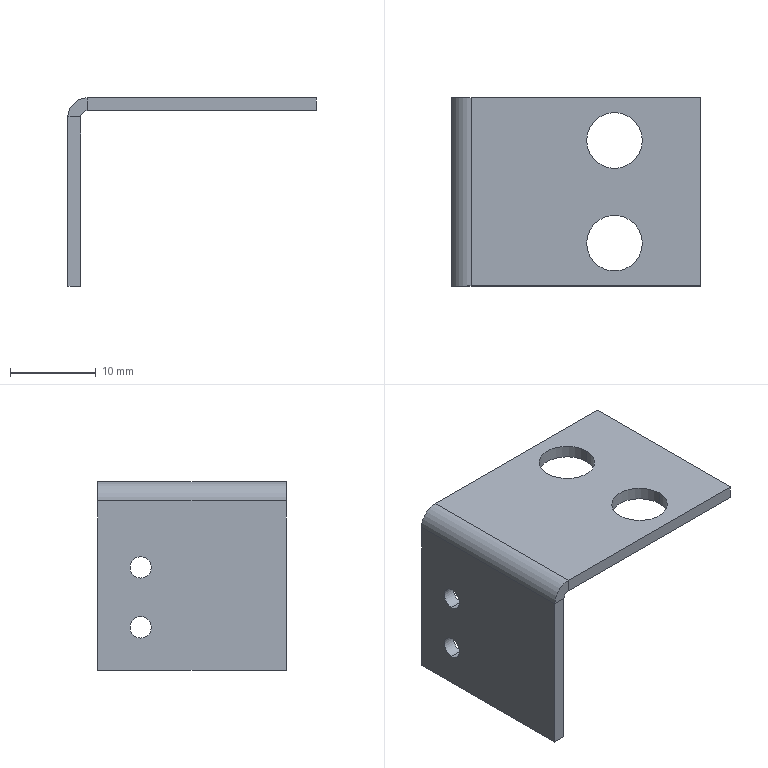Part | SolidWorks | features 3DProfileFeature 1, EdgeFlange 1, FlatPattern 1, HoleWzd 1, SMBaseFlange 1, SheetMetal 1 | 1 solid | 22 faces | box 29 x 22 x 22 mm | volume 1498 mm3 | plane 12 | cylinder 10 | commonest cylinder face diameters 2.5 x4 6.5 x4 1.473 x1 4.473 x1
STEP:
#1=CARTESIAN_POINT('',(-13.,6.,-11.25));
#2=VERTEX_POINT('',#1);
#3=CARTESIAN_POINT('',(-13.,6.,-8.75));
#4=VERTEX_POINT('',#3);
#5=CARTESIAN_POINT('',(-13.,6.,-10.));
#6=DIRECTION('',(-1.,0.,0.));
#7=DIRECTION('',(0.,0.,1.));
#8=AXIS2_PLACEMENT_3D('',#5,#6,#7);
#9=CIRCLE('',#8,1.25);
#10=EDGE_CURVE('',#2,#4,#9,.T.);
#11=ORIENTED_EDGE('',*,*,#10,.F.);
#12=CARTESIAN_POINT('',(-14.5,6.,-11.25));
#13=VERTEX_POINT('',#12);
#14=CARTESIAN_POINT('',(-14.5,6.,-11.25));
#15=DIRECTION('',(-1.,0.,0.));
#16=VECTOR('',#15,1000.);
#17=LINE('',#14,#16);
#18=EDGE_CURVE('',#2,#13,#17,.T.);
#19=ORIENTED_EDGE('',*,*,#18,.T.);
#20=CARTESIAN_POINT('',(-14.5,6.,-8.75));
#21=VERTEX_POINT('',#20);
#22=CARTESIAN_POINT('',(-14.5,6.,-10.));
#23=DIRECTION('',(-1.,0.,0.));
#24=DIRECTION('',(0.,0.,1.));
#25=AXIS2_PLACEMENT_3D('',#22,#23,#24);
#26=CIRCLE('',#25,1.25);
#27=EDGE_CURVE('',#13,#21,#26,.T.);
#28=ORIENTED_EDGE('',*,*,#27,.T.);
#29=CARTESIAN_POINT('',(-14.5,6.,-8.75));
#30=DIRECTION('',(-1.,0.,0.));
#31=VECTOR('',#30,1000.);
#32=LINE('',#29,#31);
#33=EDGE_CURVE('',#4,#21,#32,.T.);
#34=ORIENTED_EDGE('',*,*,#33,.F.);
#35=EDGE_LOOP('',(#11,#19,#28,#34));
#36=FACE_OUTER_BOUND('',#35,.T.);
#37=CARTESIAN_POINT('',(-14.5,6.,-10.));
#38=DIRECTION('',(-1.,0.,0.));
#39=DIRECTION('',(0.,0.,1.));
#40=AXIS2_PLACEMENT_3D('',#37,#38,#39);
#41=CYLINDRICAL_SURFACE('',#40,1.25);
#42=ADVANCED_FACE('',(#36),#41,.F.);
#43=CARTESIAN_POINT('',(-13.,6.,-18.25));
#44=VERTEX_POINT('',#43);
#45=CARTESIAN_POINT('',(-13.,6.,-15.75));
#46=VERTEX_POINT('',#45);
#47=CARTESIAN_POINT('',(-13.,6.,-17.));
#48=DIRECTION('',(-1.,0.,0.));
#49=DIRECTION('',(0.,0.,1.));
#50=AXIS2_PLACEMENT_3D('',#47,#48,#49);
#51=CIRCLE('',#50,1.25);
#52=EDGE_CURVE('',#44,#46,#51,.T.);
#53=ORIENTED_EDGE('',*,*,#52,.F.);
#54=CARTESIAN_POINT('',(-14.5,6.,-18.25));
#55=VERTEX_POINT('',#54);
#56=CARTESIAN_POINT('',(-14.5,6.,-18.25));
#57=DIRECTION('',(-1.,0.,0.));
#58=VECTOR('',#57,1000.);
#59=LINE('',#56,#58);
#60=EDGE_CURVE('',#44,#55,#59,.T.);
#61=ORIENTED_EDGE('',*,*,#60,.T.);
#62=CARTESIAN_POINT('',(-14.5,6.,-15.75));
#63=VERTEX_POINT('',#62);
#64=CARTESIAN_POINT('',(-14.5,6.,-17.));
#65=DIRECTION('',(-1.,0.,0.));
#66=DIRECTION('',(0.,0.,1.));
#67=AXIS2_PLACEMENT_3D('',#64,#65,#66);
#68=CIRCLE('',#67,1.25);
#69=EDGE_CURVE('',#55,#63,#68,.T.);
#70=ORIENTED_EDGE('',*,*,#69,.T.);
#71=CARTESIAN_POINT('',(-14.5,6.,-15.75));
#72=DIRECTION('',(-1.,0.,0.));
#73=VECTOR('',#72,1000.);
#74=LINE('',#71,#73);
#75=EDGE_CURVE('',#46,#63,#74,.T.);
#76=ORIENTED_EDGE('',*,*,#75,.F.);
#77=EDGE_LOOP('',(#53,#61,#70,#76));
#78=FACE_OUTER_BOUND('',#77,.T.);
#79=CARTESIAN_POINT('',(-14.5,6.,-17.));
#80=DIRECTION('',(-1.,0.,0.));
#81=DIRECTION('',(0.,0.,1.));
#82=AXIS2_PLACEMENT_3D('',#79,#80,#81);
#83=CYLINDRICAL_SURFACE('',#82,1.25);
#84=ADVANCED_FACE('',(#78),#83,.F.);
#85=CARTESIAN_POINT('',(1.25,-6.,-1.5));
#86=VERTEX_POINT('',#85);
#87=CARTESIAN_POINT('',(7.75,-6.,-1.5));
#88=VERTEX_POINT('',#87);
#89=CARTESIAN_POINT('',(4.5,-6.,-1.5));
#90=DIRECTION('',(0.,0.,1.));
#91=DIRECTION('',(1.,0.,0.));
#92=AXIS2_PLACEMENT_3D('',#89,#90,#91);
#93=CIRCLE('',#92,3.25);
#94=EDGE_CURVE('',#86,#88,#93,.T.);
#95=ORIENTED_EDGE('',*,*,#94,.F.);
#96=CARTESIAN_POINT('',(1.25,-6.,0.));
#97=VERTEX_POINT('',#96);
#98=CARTESIAN_POINT('',(1.25,-6.,-1.5));
#99=DIRECTION('',(0.,0.,1.));
#100=VECTOR('',#99,1000.);
#101=LINE('',#98,#100);
#102=EDGE_CURVE('',#86,#97,#101,.T.);
#103=ORIENTED_EDGE('',*,*,#102,.T.);
#104=CARTESIAN_POINT('',(7.75,-6.,0.));
#105=VERTEX_POINT('',#104);
#106=CARTESIAN_POINT('',(4.5,-6.,0.));
#107=DIRECTION('',(0.,0.,1.));
#108=DIRECTION('',(1.,0.,0.));
#109=AXIS2_PLACEMENT_3D('',#106,#107,#108);
#110=CIRCLE('',#109,3.25);
#111=EDGE_CURVE('',#97,#105,#110,.T.);
#112=ORIENTED_EDGE('',*,*,#111,.T.);
#113=CARTESIAN_POINT('',(7.75,-6.,-1.5));
#114=DIRECTION('',(0.,0.,1.));
#115=VECTOR('',#114,1000.);
#116=LINE('',#113,#115);
#117=EDGE_CURVE('',#88,#105,#116,.T.);
#118=ORIENTED_EDGE('',*,*,#117,.F.);
#119=EDGE_LOOP('',(#95,#103,#112,#118));
#120=FACE_OUTER_BOUND('',#119,.T.);
#121=CARTESIAN_POINT('',(4.5,-6.,-1.5));
#122=DIRECTION('',(0.,0.,1.));
#123=DIRECTION('',(1.,0.,0.));
#124=AXIS2_PLACEMENT_3D('',#121,#122,#123);
#125=CYLINDRICAL_SURFACE('',#124,3.25);
#126=ADVANCED_FACE('',(#120),#125,.F.);
#127=CARTESIAN_POINT('',(1.25,6.,-1.5));
#128=VERTEX_POINT('',#127);
#129=CARTESIAN_POINT('',(7.75,6.,-1.5));
#130=VERTEX_POINT('',#129);
#131=CARTESIAN_POINT('',(4.5,6.,-1.5));
#132=DIRECTION('',(0.,0.,1.));
#133=DIRECTION('',(1.,0.,0.));
#134=AXIS2_PLACEMENT_3D('',#131,#132,#133);
#135=CIRCLE('',#134,3.25);
#136=EDGE_CURVE('',#128,#130,#135,.T.);
#137=ORIENTED_EDGE('',*,*,#136,.F.);
#138=CARTESIAN_POINT('',(1.25,6.,0.));
#139=VERTEX_POINT('',#138);
#140=CARTESIAN_POINT('',(1.25,6.,-1.5));
#141=DIRECTION('',(0.,0.,1.));
#142=VECTOR('',#141,1000.);
#143=LINE('',#140,#142);
#144=EDGE_CURVE('',#128,#139,#143,.T.);
#145=ORIENTED_EDGE('',*,*,#144,.T.);
#146=CARTESIAN_POINT('',(7.75,6.,0.));
#147=VERTEX_POINT('',#146);
#148=CARTESIAN_POINT('',(4.5,6.,0.));
#149=DIRECTION('',(0.,0.,1.));
#150=DIRECTION('',(1.,0.,0.));
#151=AXIS2_PLACEMENT_3D('',#148,#149,#150);
#152=CIRCLE('',#151,3.25);
#153=EDGE_CURVE('',#139,#147,#152,.T.);
#154=ORIENTED_EDGE('',*,*,#153,.T.);
#155=CARTESIAN_POINT('',(7.75,6.,-1.5));
#156=DIRECTION('',(0.,0.,1.));
#157=VECTOR('',#156,1000.);
#158=LINE('',#155,#157);
#159=EDGE_CURVE('',#130,#147,#158,.T.);
#160=ORIENTED_EDGE('',*,*,#159,.F.);
#161=EDGE_LOOP('',(#137,#145,#154,#160));
#162=FACE_OUTER_BOUND('',#161,.T.);
#163=CARTESIAN_POINT('',(4.5,6.,-1.5));
#164=DIRECTION('',(0.,0.,1.));
#165=DIRECTION('',(1.,0.,0.));
#166=AXIS2_PLACEMENT_3D('',#163,#164,#165);
#167=CYLINDRICAL_SURFACE('',#166,3.25);
#168=ADVANCED_FACE('',(#162),#167,.F.);
#169=CARTESIAN_POINT('',(14.5,11.,-1.5));
#170=VERTEX_POINT('',#169);
#171=CARTESIAN_POINT('',(-12.263,11.,-1.5));
#172=VERTEX_POINT('',#171);
#173=CARTESIAN_POINT('',(-14.5,11.,-1.5));
#174=DIRECTION('',(-1.,0.,0.));
#175=VECTOR('',#174,1000.);
#176=LINE('',#173,#175);
#177=EDGE_CURVE('',#170,#172,#176,.T.);
#178=ORIENTED_EDGE('',*,*,#177,.T.);
#179=CARTESIAN_POINT('',(-12.263,11.,0.));
#180=VERTEX_POINT('',#179);
#181=CARTESIAN_POINT('',(-12.263,11.,-1.5));
#182=DIRECTION('',(0.,0.,1.));
#183=VECTOR('',#182,1000.);
#184=LINE('',#181,#183);
#185=EDGE_CURVE('',#172,#180,#184,.T.);
#186=ORIENTED_EDGE('',*,*,#185,.T.);
#187=CARTESIAN_POINT('',(14.5,11.,0.));
#188=VERTEX_POINT('',#187);
#189=CARTESIAN_POINT('',(-14.5,11.,0.));
#190=DIRECTION('',(-1.,0.,0.));
#191=VECTOR('',#190,1000.);
#192=LINE('',#189,#191);
#193=EDGE_CURVE('',#188,#180,#192,.T.);
#194=ORIENTED_EDGE('',*,*,#193,.F.);
#195=CARTESIAN_POINT('',(14.5,11.,-1.5));
#196=DIRECTION('',(0.,0.,1.));
#197=VECTOR('',#196,1000.);
#198=LINE('',#195,#197);
#199=EDGE_CURVE('',#170,#188,#198,.T.);
#200=ORIENTED_EDGE('',*,*,#199,.F.);
#201=EDGE_LOOP('',(#178,#186,#194,#200));
#202=FACE_OUTER_BOUND('',#201,.T.);
#203=CARTESIAN_POINT('',(-14.5,11.,-1.5));
#204=DIRECTION('',(0.,1.,0.));
#205=DIRECTION('',(0.,0.,1.));
#206=AXIS2_PLACEMENT_3D('',#203,#204,#205);
#207=PLANE('',#206);
#208=ADVANCED_FACE('',(#202),#207,.T.);
#209=CARTESIAN_POINT('',(4.5,6.,-1.5));
#210=DIRECTION('',(0.,0.,1.));
#211=DIRECTION('',(1.,0.,0.));
#212=AXIS2_PLACEMENT_3D('',#209,#210,#211);
#213=CIRCLE('',#212,3.25);
#214=EDGE_CURVE('',#130,#128,#213,.T.);
#215=ORIENTED_EDGE('',*,*,#214,.T.);
#216=ORIENTED_EDGE('',*,*,#136,.T.);
#217=EDGE_LOOP('',(#215,#216));
#218=FACE_BOUND('',#217,.T.);
#219=CARTESIAN_POINT('',(4.5,-6.,-1.5));
#220=DIRECTION('',(0.,0.,1.));
#221=DIRECTION('',(1.,0.,0.));
#222=AXIS2_PLACEMENT_3D('',#219,#220,#221);
#223=CIRCLE('',#222,3.25);
#224=EDGE_CURVE('',#88,#86,#223,.T.);
#225=ORIENTED_EDGE('',*,*,#224,.T.);
#226=ORIENTED_EDGE('',*,*,#94,.T.);
#227=EDGE_LOOP('',(#225,#226));
#228=FACE_BOUND('',#227,.T.);
#229=CARTESIAN_POINT('',(-12.263,-11.,-1.5));
#230=VERTEX_POINT('',#229);
#231=CARTESIAN_POINT('',(-12.263,11.,-1.5));
#232=DIRECTION('',(0.,-1.,0.));
#233=VECTOR('',#232,1000.);
#234=LINE('',#231,#233);
#235=EDGE_CURVE('',#172,#230,#234,.T.);
#236=ORIENTED_EDGE('',*,*,#235,.F.);
#237=ORIENTED_EDGE('',*,*,#177,.F.);
#238=CARTESIAN_POINT('',(14.5,-11.,-1.5));
#239=VERTEX_POINT('',#238);
#240=CARTESIAN_POINT('',(14.5,11.,-1.5));
#241=DIRECTION('',(0.,1.,0.));
#242=VECTOR('',#241,1000.);
#243=LINE('',#240,#242);
#244=EDGE_CURVE('',#239,#170,#243,.T.);
#245=ORIENTED_EDGE('',*,*,#244,.F.);
#246=CARTESIAN_POINT('',(-14.5,-11.,-1.5));
#247=DIRECTION('',(1.,0.,0.));
#248=VECTOR('',#247,1000.);
#249=LINE('',#246,#248);
#250=EDGE_CURVE('',#230,#239,#249,.T.);
#251=ORIENTED_EDGE('',*,*,#250,.F.);
#252=EDGE_LOOP('',(#236,#237,#245,#251));
#253=FACE_OUTER_BOUND('',#252,.T.);
#254=CARTESIAN_POINT('',(0.,0.,-1.5));
#255=DIRECTION('',(0.,0.,1.));
#256=DIRECTION('',(1.,0.,0.));
#257=AXIS2_PLACEMENT_3D('',#254,#255,#256);
#258=PLANE('',#257);
#259=ADVANCED_FACE('',(#218,#228,#253),#258,.F.);
#260=CARTESIAN_POINT('',(4.5,6.,0.));
#261=DIRECTION('',(0.,0.,1.));
#262=DIRECTION('',(1.,0.,0.));
#263=AXIS2_PLACEMENT_3D('',#260,#261,#262);
#264=CIRCLE('',#263,3.25);
#265=EDGE_CURVE('',#147,#139,#264,.T.);
#266=ORIENTED_EDGE('',*,*,#265,.F.);
#267=ORIENTED_EDGE('',*,*,#153,.F.);
#268=EDGE_LOOP('',(#266,#267));
#269=FACE_BOUND('',#268,.T.);
#270=CARTESIAN_POINT('',(4.5,-6.,0.));
#271=DIRECTION('',(0.,0.,1.));
#272=DIRECTION('',(1.,0.,0.));
#273=AXIS2_PLACEMENT_3D('',#270,#271,#272);
#274=CIRCLE('',#273,3.25);
#275=EDGE_CURVE('',#105,#97,#274,.T.);
#276=ORIENTED_EDGE('',*,*,#275,.F.);
#277=ORIENTED_EDGE('',*,*,#111,.F.);
#278=EDGE_LOOP('',(#276,#277));
#279=FACE_BOUND('',#278,.T.);
#280=ORIENTED_EDGE('',*,*,#193,.T.);
#281=CARTESIAN_POINT('',(-12.263,-11.,0.));
#282=VERTEX_POINT('',#281);
#283=CARTESIAN_POINT('',(-12.263,11.,0.));
#284=DIRECTION('',(0.,-1.,0.));
#285=VECTOR('',#284,1000.);
#286=LINE('',#283,#285);
#287=EDGE_CURVE('',#180,#282,#286,.T.);
#288=ORIENTED_EDGE('',*,*,#287,.T.);
#289=CARTESIAN_POINT('',(14.5,-11.,0.));
#290=VERTEX_POINT('',#289);
#291=CARTESIAN_POINT('',(-14.5,-11.,0.));
#292=DIRECTION('',(1.,0.,0.));
#293=VECTOR('',#292,1000.);
#294=LINE('',#291,#293);
#295=EDGE_CURVE('',#282,#290,#294,.T.);
#296=ORIENTED_EDGE('',*,*,#295,.T.);
#297=CARTESIAN_POINT('',(14.5,11.,0.));
#298=DIRECTION('',(0.,1.,0.));
#299=VECTOR('',#298,1000.);
#300=LINE('',#297,#299);
#301=EDGE_CURVE('',#290,#188,#300,.T.);
#302=ORIENTED_EDGE('',*,*,#301,.T.);
#303=EDGE_LOOP('',(#280,#288,#296,#302));
#304=FACE_OUTER_BOUND('',#303,.T.);
#305=CARTESIAN_POINT('',(0.,0.,0.));
#306=DIRECTION('',(0.,0.,1.));
#307=DIRECTION('',(1.,0.,0.));
#308=AXIS2_PLACEMENT_3D('',#305,#306,#307);
#309=PLANE('',#308);
#310=ADVANCED_FACE('',(#269,#279,#304),#309,.T.);
#311=ORIENTED_EDGE('',*,*,#301,.F.);
#312=CARTESIAN_POINT('',(14.5,-11.,-1.5));
#313=DIRECTION('',(0.,0.,1.));
#314=VECTOR('',#313,1000.);
#315=LINE('',#312,#314);
#316=EDGE_CURVE('',#239,#290,#315,.T.);
#317=ORIENTED_EDGE('',*,*,#316,.F.);
#318=ORIENTED_EDGE('',*,*,#244,.T.);
#319=ORIENTED_EDGE('',*,*,#199,.T.);
#320=EDGE_LOOP('',(#311,#317,#318,#319));
#321=FACE_OUTER_BOUND('',#320,.T.);
#322=CARTESIAN_POINT('',(14.5,11.,-1.5));
#323=DIRECTION('',(1.,0.,0.));
#324=DIRECTION('',(0.,1.,0.));
#325=AXIS2_PLACEMENT_3D('',#322,#323,#324);
#326=PLANE('',#325);
#327=ADVANCED_FACE('',(#321),#326,.T.);
#328=CARTESIAN_POINT('',(-12.263,-11.,-1.5));
#329=DIRECTION('',(0.,0.,1.));
#330=VECTOR('',#329,1000.);
#331=LINE('',#328,#330);
#332=EDGE_CURVE('',#230,#282,#331,.T.);
#333=ORIENTED_EDGE('',*,*,#332,.F.);
#334=ORIENTED_EDGE('',*,*,#250,.T.);
#335=ORIENTED_EDGE('',*,*,#316,.T.);
#336=ORIENTED_EDGE('',*,*,#295,.F.);
#337=EDGE_LOOP('',(#333,#334,#335,#336));
#338=FACE_OUTER_BOUND('',#337,.T.);
#339=CARTESIAN_POINT('',(-14.5,-11.,-1.5));
#340=DIRECTION('',(0.,-1.,0.));
#341=DIRECTION('',(0.,0.,-1.));
#342=AXIS2_PLACEMENT_3D('',#339,#340,#341);
#343=PLANE('',#342);
#344=ADVANCED_FACE('',(#338),#343,.T.);
#345=ORIENTED_EDGE('',*,*,#144,.F.);
#346=ORIENTED_EDGE('',*,*,#214,.F.);
#347=ORIENTED_EDGE('',*,*,#159,.T.);
#348=ORIENTED_EDGE('',*,*,#265,.T.);
#349=EDGE_LOOP('',(#345,#346,#347,#348));
#350=FACE_OUTER_BOUND('',#349,.T.);
#351=CARTESIAN_POINT('',(4.5,6.,-1.5));
#352=DIRECTION('',(0.,0.,1.));
#353=DIRECTION('',(1.,0.,0.));
#354=AXIS2_PLACEMENT_3D('',#351,#352,#353);
#355=CYLINDRICAL_SURFACE('',#354,3.25);
#356=ADVANCED_FACE('',(#350),#355,.F.);
#357=ORIENTED_EDGE('',*,*,#102,.F.);
#358=ORIENTED_EDGE('',*,*,#224,.F.);
#359=ORIENTED_EDGE('',*,*,#117,.T.);
#360=ORIENTED_EDGE('',*,*,#275,.T.);
#361=EDGE_LOOP('',(#357,#358,#359,#360));
#362=FACE_OUTER_BOUND('',#361,.T.);
#363=CARTESIAN_POINT('',(4.5,-6.,-1.5));
#364=DIRECTION('',(0.,0.,1.));
#365=DIRECTION('',(1.,0.,0.));
#366=AXIS2_PLACEMENT_3D('',#363,#364,#365);
#367=CYLINDRICAL_SURFACE('',#366,3.25);
#368=ADVANCED_FACE('',(#362),#367,.F.);
#369=CARTESIAN_POINT('',(-13.,-11.,-2.237));
#370=VERTEX_POINT('',#369);
#371=CARTESIAN_POINT('',(-14.5,-11.,-2.237));
#372=VERTEX_POINT('',#371);
#373=CARTESIAN_POINT('',(-14.5,-11.,-2.237));
#374=DIRECTION('',(-1.,0.,0.));
#375=VECTOR('',#374,1000.);
#376=LINE('',#373,#375);
#377=EDGE_CURVE('',#370,#372,#376,.T.);
#378=ORIENTED_EDGE('',*,*,#377,.F.);
#379=CARTESIAN_POINT('',(-12.263,-11.,-2.237));
#380=DIRECTION('',(0.,-1.,0.));
#381=DIRECTION('',(0.,0.,1.));
#382=AXIS2_PLACEMENT_3D('',#379,#380,#381);
#383=CIRCLE('',#382,0.7366);
#384=EDGE_CURVE('',#230,#370,#383,.T.);
#385=ORIENTED_EDGE('',*,*,#384,.F.);
#386=ORIENTED_EDGE('',*,*,#332,.T.);
#387=CARTESIAN_POINT('',(-12.263,-11.,-2.237));
#388=DIRECTION('',(0.,-1.,0.));
#389=DIRECTION('',(0.,0.,1.));
#390=AXIS2_PLACEMENT_3D('',#387,#388,#389);
#391=CIRCLE('',#390,2.237);
#392=EDGE_CURVE('',#282,#372,#391,.T.);
#393=ORIENTED_EDGE('',*,*,#392,.T.);
#394=EDGE_LOOP('',(#378,#385,#386,#393));
#395=FACE_OUTER_BOUND('',#394,.T.);
#396=CARTESIAN_POINT('',(-12.263,-11.,-2.237));
#397=DIRECTION('',(0.,-1.,0.));
#398=DIRECTION('',(0.,0.,-1.));
#399=AXIS2_PLACEMENT_3D('',#396,#397,#398);
#400=PLANE('',#399);
#401=ADVANCED_FACE('',(#395),#400,.T.);
#402=CARTESIAN_POINT('',(-13.,11.,-2.237));
#403=VERTEX_POINT('',#402);
#404=CARTESIAN_POINT('',(-12.263,11.,-2.237));
#405=DIRECTION('',(0.,1.,0.));
#406=DIRECTION('',(0.,0.,1.));
#407=AXIS2_PLACEMENT_3D('',#404,#405,#406);
#408=CIRCLE('',#407,0.7366);
#409=EDGE_CURVE('',#403,#172,#408,.T.);
#410=ORIENTED_EDGE('',*,*,#409,.F.);
#411=CARTESIAN_POINT('',(-14.5,11.,-2.237));
#412=VERTEX_POINT('',#411);
#413=CARTESIAN_POINT('',(-13.,11.,-2.237));
#414=DIRECTION('',(-1.,0.,0.));
#415=VECTOR('',#414,1000.);
#416=LINE('',#413,#415);
#417=EDGE_CURVE('',#403,#412,#416,.T.);
#418=ORIENTED_EDGE('',*,*,#417,.T.);
#419=CARTESIAN_POINT('',(-12.263,11.,-2.237));
#420=DIRECTION('',(0.,1.,0.));
#421=DIRECTION('',(0.,0.,1.));
#422=AXIS2_PLACEMENT_3D('',#419,#420,#421);
#423=CIRCLE('',#422,2.237);
#424=EDGE_CURVE('',#412,#180,#423,.T.);
#425=ORIENTED_EDGE('',*,*,#424,.T.);
#426=ORIENTED_EDGE('',*,*,#185,.F.);
#427=EDGE_LOOP('',(#410,#418,#425,#426));
#428=FACE_OUTER_BOUND('',#427,.T.);
#429=CARTESIAN_POINT('',(-12.263,11.,-2.237));
#430=DIRECTION('',(0.,-1.,0.));
#431=DIRECTION('',(0.,0.,-1.));
#432=AXIS2_PLACEMENT_3D('',#429,#430,#431);
#433=PLANE('',#432);
#434=ADVANCED_FACE('',(#428),#433,.F.);
#435=ORIENTED_EDGE('',*,*,#287,.F.);
#436=ORIENTED_EDGE('',*,*,#424,.F.);
#437=CARTESIAN_POINT('',(-14.5,0.,-2.237));
#438=DIRECTION('',(0.,1.,0.));
#439=VECTOR('',#438,1000.);
#440=LINE('',#437,#439);
#441=EDGE_CURVE('',#372,#412,#440,.T.);
#442=ORIENTED_EDGE('',*,*,#441,.F.);
#443=ORIENTED_EDGE('',*,*,#392,.F.);
#444=EDGE_LOOP('',(#435,#436,#442,#443));
#445=FACE_OUTER_BOUND('',#444,.T.);
#446=CARTESIAN_POINT('',(-12.263,11.,-2.237));
#447=DIRECTION('',(0.,1.,0.));
#448=DIRECTION('',(-1.,0.,0.));
#449=AXIS2_PLACEMENT_3D('',#446,#447,#448);
#450=CYLINDRICAL_SURFACE('',#449,2.237);
#451=ADVANCED_FACE('',(#445),#450,.T.);
#452=ORIENTED_EDGE('',*,*,#235,.T.);
#453=ORIENTED_EDGE('',*,*,#384,.T.);
#454=CARTESIAN_POINT('',(-13.,-11.,-2.237));
#455=DIRECTION('',(0.,1.,0.));
#456=VECTOR('',#455,1000.);
#457=LINE('',#454,#456);
#458=EDGE_CURVE('',#370,#403,#457,.T.);
#459=ORIENTED_EDGE('',*,*,#458,.T.);
#460=ORIENTED_EDGE('',*,*,#409,.T.);
#461=EDGE_LOOP('',(#452,#453,#459,#460));
#462=FACE_OUTER_BOUND('',#461,.T.);
#463=CARTESIAN_POINT('',(-12.263,11.,-2.237));
#464=DIRECTION('',(0.,1.,0.));
#465=DIRECTION('',(-1.,0.,0.));
#466=AXIS2_PLACEMENT_3D('',#463,#464,#465);
#467=CYLINDRICAL_SURFACE('',#466,0.7366);
#468=ADVANCED_FACE('',(#462),#467,.F.);
#469=CARTESIAN_POINT('',(-14.5,11.,-22.));
#470=VERTEX_POINT('',#469);
#471=CARTESIAN_POINT('',(-14.5,11.,-1.5));
#472=DIRECTION('',(0.,0.,1.));
#473=VECTOR('',#472,1000.);
#474=LINE('',#471,#473);
#475=EDGE_CURVE('',#470,#412,#474,.T.);
#476=ORIENTED_EDGE('',*,*,#475,.T.);
#477=ORIENTED_EDGE('',*,*,#417,.F.);
#478=CARTESIAN_POINT('',(-13.,11.,-22.));
#479=VERTEX_POINT('',#478);
#480=CARTESIAN_POINT('',(-13.,11.,0.));
#481=DIRECTION('',(0.,0.,1.));
#482=VECTOR('',#481,1000.);
#483=LINE('',#480,#482);
#484=EDGE_CURVE('',#479,#403,#483,.T.);
#485=ORIENTED_EDGE('',*,*,#484,.F.);
#486=CARTESIAN_POINT('',(-14.5,11.,-22.));
#487=DIRECTION('',(1.,0.,0.));
#488=VECTOR('',#487,1000.);
#489=LINE('',#486,#488);
#490=EDGE_CURVE('',#470,#479,#489,.T.);
#491=ORIENTED_EDGE('',*,*,#490,.F.);
#492=EDGE_LOOP('',(#476,#477,#485,#491));
#493=FACE_OUTER_BOUND('',#492,.T.);
#494=CARTESIAN_POINT('',(-14.5,11.,-1.5));
#495=DIRECTION('',(0.,1.,0.));
#496=DIRECTION('',(-1.,0.,0.));
#497=AXIS2_PLACEMENT_3D('',#494,#495,#496);
#498=PLANE('',#497);
#499=ADVANCED_FACE('',(#493),#498,.T.);
#500=CARTESIAN_POINT('',(-13.,-11.,-22.));
#501=VERTEX_POINT('',#500);
#502=CARTESIAN_POINT('',(-13.,-11.,0.));
#503=DIRECTION('',(0.,0.,-1.));
#504=VECTOR('',#503,1000.);
#505=LINE('',#502,#504);
#506=EDGE_CURVE('',#370,#501,#505,.T.);
#507=ORIENTED_EDGE('',*,*,#506,.F.);
#508=ORIENTED_EDGE('',*,*,#377,.T.);
#509=CARTESIAN_POINT('',(-14.5,-11.,-22.));
#510=VERTEX_POINT('',#509);
#511=CARTESIAN_POINT('',(-14.5,-11.,-22.));
#512=DIRECTION('',(0.,0.,-1.));
#513=VECTOR('',#512,1000.);
#514=LINE('',#511,#513);
#515=EDGE_CURVE('',#372,#510,#514,.T.);
#516=ORIENTED_EDGE('',*,*,#515,.T.);
#517=CARTESIAN_POINT('',(-14.5,-11.,-22.));
#518=DIRECTION('',(1.,0.,0.));
#519=VECTOR('',#518,1000.);
#520=LINE('',#517,#519);
#521=EDGE_CURVE('',#510,#501,#520,.T.);
#522=ORIENTED_EDGE('',*,*,#521,.T.);
#523=EDGE_LOOP('',(#507,#508,#516,#522));
#524=FACE_OUTER_BOUND('',#523,.T.);
#525=CARTESIAN_POINT('',(-14.5,-11.,-22.));
#526=DIRECTION('',(0.,-1.,0.));
#527=DIRECTION('',(1.,0.,0.));
#528=AXIS2_PLACEMENT_3D('',#525,#526,#527);
#529=PLANE('',#528);
#530=ADVANCED_FACE('',(#524),#529,.T.);
#531=CARTESIAN_POINT('',(-14.5,6.,-10.));
#532=DIRECTION('',(-1.,0.,0.));
#533=DIRECTION('',(0.,0.,1.));
#534=AXIS2_PLACEMENT_3D('',#531,#532,#533);
#535=CIRCLE('',#534,1.25);
#536=EDGE_CURVE('',#21,#13,#535,.T.);
#537=ORIENTED_EDGE('',*,*,#536,.F.);
#538=ORIENTED_EDGE('',*,*,#27,.F.);
#539=EDGE_LOOP('',(#537,#538));
#540=FACE_BOUND('',#539,.T.);
#541=CARTESIAN_POINT('',(-14.5,6.,-17.));
#542=DIRECTION('',(-1.,0.,0.));
#543=DIRECTION('',(0.,0.,1.));
#544=AXIS2_PLACEMENT_3D('',#541,#542,#543);
#545=CIRCLE('',#544,1.25);
#546=EDGE_CURVE('',#63,#55,#545,.T.);
#547=ORIENTED_EDGE('',*,*,#546,.F.);
#548=ORIENTED_EDGE('',*,*,#69,.F.);
#549=EDGE_LOOP('',(#547,#548));
#550=FACE_BOUND('',#549,.T.);
#551=ORIENTED_EDGE('',*,*,#515,.F.);
#552=ORIENTED_EDGE('',*,*,#441,.T.);
#553=ORIENTED_EDGE('',*,*,#475,.F.);
#554=CARTESIAN_POINT('',(-14.5,11.,-22.));
#555=DIRECTION('',(0.,1.,0.));
#556=VECTOR('',#555,1000.);
#557=LINE('',#554,#556);
#558=EDGE_CURVE('',#510,#470,#557,.T.);
#559=ORIENTED_EDGE('',*,*,#558,.F.);
#560=EDGE_LOOP('',(#551,#552,#553,#559));
#561=FACE_OUTER_BOUND('',#560,.T.);
#562=CARTESIAN_POINT('',(-14.5,0.,0.));
#563=DIRECTION('',(-1.,0.,0.));
#564=DIRECTION('',(0.,0.,1.));
#565=AXIS2_PLACEMENT_3D('',#562,#563,#564);
#566=PLANE('',#565);
#567=ADVANCED_FACE('',(#540,#550,#561),#566,.T.);
#568=CARTESIAN_POINT('',(-13.,6.,-10.));
#569=DIRECTION('',(-1.,0.,0.));
#570=DIRECTION('',(0.,0.,1.));
#571=AXIS2_PLACEMENT_3D('',#568,#569,#570);
#572=CIRCLE('',#571,1.25);
#573=EDGE_CURVE('',#4,#2,#572,.T.);
#574=ORIENTED_EDGE('',*,*,#573,.T.);
#575=ORIENTED_EDGE('',*,*,#10,.T.);
#576=EDGE_LOOP('',(#574,#575));
#577=FACE_BOUND('',#576,.T.);
#578=CARTESIAN_POINT('',(-13.,6.,-17.));
#579=DIRECTION('',(-1.,0.,0.));
#580=DIRECTION('',(0.,0.,1.));
#581=AXIS2_PLACEMENT_3D('',#578,#579,#580);
#582=CIRCLE('',#581,1.25);
#583=EDGE_CURVE('',#46,#44,#582,.T.);
#584=ORIENTED_EDGE('',*,*,#583,.T.);
#585=ORIENTED_EDGE('',*,*,#52,.T.);
#586=EDGE_LOOP('',(#584,#585));
#587=FACE_BOUND('',#586,.T.);
#588=ORIENTED_EDGE('',*,*,#458,.F.);
#589=ORIENTED_EDGE('',*,*,#506,.T.);
#590=CARTESIAN_POINT('',(-13.,0.,-22.));
#591=DIRECTION('',(0.,1.,0.));
#592=VECTOR('',#591,1000.);
#593=LINE('',#590,#592);
#594=EDGE_CURVE('',#501,#479,#593,.T.);
#595=ORIENTED_EDGE('',*,*,#594,.T.);
#596=ORIENTED_EDGE('',*,*,#484,.T.);
#597=EDGE_LOOP('',(#588,#589,#595,#596));
#598=FACE_OUTER_BOUND('',#597,.T.);
#599=CARTESIAN_POINT('',(-13.,0.,0.));
#600=DIRECTION('',(-1.,0.,0.));
#601=DIRECTION('',(0.,0.,1.));
#602=AXIS2_PLACEMENT_3D('',#599,#600,#601);
#603=PLANE('',#602);
#604=ADVANCED_FACE('',(#577,#587,#598),#603,.F.);
#605=ORIENTED_EDGE('',*,*,#594,.F.);
#606=ORIENTED_EDGE('',*,*,#521,.F.);
#607=ORIENTED_EDGE('',*,*,#558,.T.);
#608=ORIENTED_EDGE('',*,*,#490,.T.);
#609=EDGE_LOOP('',(#605,#606,#607,#608));
#610=FACE_OUTER_BOUND('',#609,.T.);
#611=CARTESIAN_POINT('',(-14.5,11.,-22.));
#612=DIRECTION('',(0.,0.,-1.));
#613=DIRECTION('',(-1.,0.,0.));
#614=AXIS2_PLACEMENT_3D('',#611,#612,#613);
#615=PLANE('',#614);
#616=ADVANCED_FACE('',(#610),#615,.T.);
#617=ORIENTED_EDGE('',*,*,#60,.F.);
#618=ORIENTED_EDGE('',*,*,#583,.F.);
#619=ORIENTED_EDGE('',*,*,#75,.T.);
#620=ORIENTED_EDGE('',*,*,#546,.T.);
#621=EDGE_LOOP('',(#617,#618,#619,#620));
#622=FACE_OUTER_BOUND('',#621,.T.);
#623=CARTESIAN_POINT('',(-14.5,6.,-17.));
#624=DIRECTION('',(-1.,0.,0.));
#625=DIRECTION('',(0.,0.,1.));
#626=AXIS2_PLACEMENT_3D('',#623,#624,#625);
#627=CYLINDRICAL_SURFACE('',#626,1.25);
#628=ADVANCED_FACE('',(#622),#627,.F.);
#629=ORIENTED_EDGE('',*,*,#18,.F.);
#630=ORIENTED_EDGE('',*,*,#573,.F.);
#631=ORIENTED_EDGE('',*,*,#33,.T.);
#632=ORIENTED_EDGE('',*,*,#536,.T.);
#633=EDGE_LOOP('',(#629,#630,#631,#632));
#634=FACE_OUTER_BOUND('',#633,.T.);
#635=CARTESIAN_POINT('',(-14.5,6.,-10.));
#636=DIRECTION('',(-1.,0.,0.));
#637=DIRECTION('',(0.,0.,1.));
#638=AXIS2_PLACEMENT_3D('',#635,#636,#637);
#639=CYLINDRICAL_SURFACE('',#638,1.25);
#640=ADVANCED_FACE('',(#634),#639,.F.);
#641=CLOSED_SHELL('',(#42,#84,#126,#168,#208,#259,#310,#327,#344,#356,#368,#401,#434,#451,#468,#499,#530,#567,#604,#616,#628,#640));
#642=MANIFOLD_SOLID_BREP('',#641);
#643=CARTESIAN_POINT('',(0.,0.,0.));
#644=DIRECTION('',(0.,0.,1.));
#645=DIRECTION('',(1.,0.,0.));
#646=AXIS2_PLACEMENT_3D('',#643,#644,#645);
#647=(LENGTH_UNIT()NAMED_UNIT(*)SI_UNIT(.MILLI.,.METRE.));
#648=UNCERTAINTY_MEASURE_WITH_UNIT(LENGTH_MEASURE(0.00001),#647,'','');
#649=(NAMED_UNIT(*)PLANE_ANGLE_UNIT()SI_UNIT($,.RADIAN.));
#650=(NAMED_UNIT(*)SI_UNIT($,.STERADIAN.)SOLID_ANGLE_UNIT());
#651=(GEOMETRIC_REPRESENTATION_CONTEXT(3)GLOBAL_UNCERTAINTY_ASSIGNED_CONTEXT((#648))GLOBAL_UNIT_ASSIGNED_CONTEXT((#647,#649,#650))REPRESENTATION_CONTEXT('',''));
#652=ADVANCED_BREP_SHAPE_REPRESENTATION('',(#642,#646),#651);